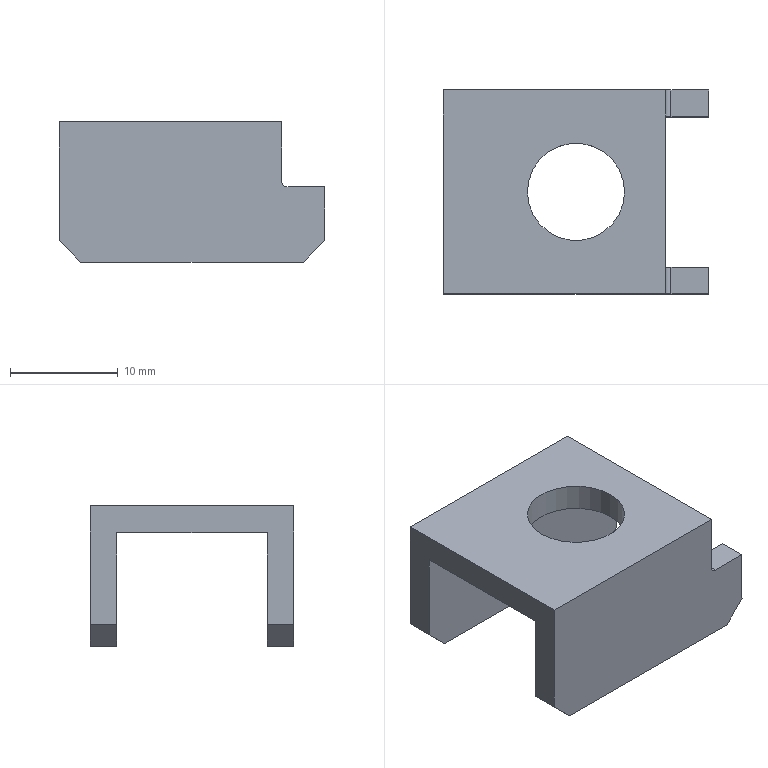Part | STEP file | gslz 2016.10.28-6_id814_x_t | 1 solid | 21 faces | box 24.6 x 18.9 x 13 mm | volume 2016 mm3 | plane 18 | cylinder 3 | commonest cylinder face diameters 1 x2 9 x1
STEP:
#1=CARTESIAN_POINT('',(165.6,245.,127.492));
#2=VERTEX_POINT('',#1);
#3=CARTESIAN_POINT('',(161.1,245.,127.492));
#4=DIRECTION('',(0.,0.,-1.));
#5=DIRECTION('',(1.,0.,0.));
#6=AXIS2_PLACEMENT_3D('',#3,#4,#5);
#7=CIRCLE('',#6,4.5);
#8=EDGE_CURVE('',#2,#2,#7,.T.);
#9=ORIENTED_EDGE('',*,*,#8,.T.);
#10=EDGE_LOOP('',(#9));
#11=FACE_BOUND('',#10,.T.);
#12=CARTESIAN_POINT('',(156.6,245.,129.992));
#13=VERTEX_POINT('',#12);
#14=CARTESIAN_POINT('',(161.1,245.,129.992));
#15=DIRECTION('',(0.,0.,-1.));
#16=DIRECTION('',(-1.,0.,0.));
#17=AXIS2_PLACEMENT_3D('',#14,#15,#16);
#18=CIRCLE('',#17,4.5);
#19=EDGE_CURVE('',#13,#13,#18,.T.);
#20=ORIENTED_EDGE('',*,*,#19,.F.);
#21=EDGE_LOOP('',(#20));
#22=FACE_BOUND('',#21,.T.);
#23=CARTESIAN_POINT('',(161.1,245.,233.066));
#24=DIRECTION('',(0.,0.,-1.));
#25=DIRECTION('',(-1.,0.,0.));
#26=AXIS2_PLACEMENT_3D('',#23,#24,#25);
#27=CYLINDRICAL_SURFACE('',#26,4.5);
#28=ADVANCED_FACE('',(#11,#22),#27,.F.);
#29=ORIENTED_EDGE('',*,*,#8,.F.);
#30=EDGE_LOOP('',(#29));
#31=FACE_BOUND('',#30,.T.);
#32=CARTESIAN_POINT('',(148.8,251.95,127.492));
#33=VERTEX_POINT('',#32);
#34=CARTESIAN_POINT('',(169.4,251.95,127.492));
#35=VERTEX_POINT('',#34);
#36=CARTESIAN_POINT('',(148.8,251.95,127.492));
#37=DIRECTION('',(1.,0.,0.));
#38=VECTOR('',#37,1.);
#39=LINE('',#36,#38);
#40=EDGE_CURVE('',#33,#35,#39,.T.);
#41=ORIENTED_EDGE('',*,*,#40,.T.);
#42=CARTESIAN_POINT('',(169.4,238.05,127.492));
#43=VERTEX_POINT('',#42);
#44=CARTESIAN_POINT('',(169.4,224.55,127.492));
#45=DIRECTION('',(0.,-1.,0.));
#46=VECTOR('',#45,1.);
#47=LINE('',#44,#46);
#48=EDGE_CURVE('',#35,#43,#47,.T.);
#49=ORIENTED_EDGE('',*,*,#48,.T.);
#50=CARTESIAN_POINT('',(148.8,238.05,127.492));
#51=VERTEX_POINT('',#50);
#52=CARTESIAN_POINT('',(173.4,238.05,127.492));
#53=DIRECTION('',(-1.,0.,0.));
#54=VECTOR('',#53,1.);
#55=LINE('',#52,#54);
#56=EDGE_CURVE('',#43,#51,#55,.T.);
#57=ORIENTED_EDGE('',*,*,#56,.T.);
#58=CARTESIAN_POINT('',(148.8,238.05,127.492));
#59=DIRECTION('',(0.,1.,0.));
#60=VECTOR('',#59,1.);
#61=LINE('',#58,#60);
#62=EDGE_CURVE('',#51,#33,#61,.T.);
#63=ORIENTED_EDGE('',*,*,#62,.T.);
#64=EDGE_LOOP('',(#41,#49,#57,#63));
#65=FACE_BOUND('',#64,.T.);
#66=CARTESIAN_POINT('',(173.4,251.95,127.492));
#67=DIRECTION('',(0.,0.,1.));
#68=DIRECTION('',(-1.,0.,0.));
#69=AXIS2_PLACEMENT_3D('',#66,#67,#68);
#70=PLANE('',#69);
#71=ADVANCED_FACE('',(#31,#65),#70,.F.);
#72=CARTESIAN_POINT('',(148.8,254.45,129.992));
#73=VERTEX_POINT('',#72);
#74=CARTESIAN_POINT('',(169.4,254.45,129.992));
#75=VERTEX_POINT('',#74);
#76=CARTESIAN_POINT('',(151.8,254.45,129.992));
#77=DIRECTION('',(1.,0.,0.));
#78=VECTOR('',#77,1.);
#79=LINE('',#76,#78);
#80=EDGE_CURVE('',#73,#75,#79,.T.);
#81=ORIENTED_EDGE('',*,*,#80,.F.);
#82=CARTESIAN_POINT('',(148.8,235.55,129.992));
#83=VERTEX_POINT('',#82);
#84=CARTESIAN_POINT('',(148.8,224.55,129.992));
#85=DIRECTION('',(0.,1.,0.));
#86=VECTOR('',#85,1.);
#87=LINE('',#84,#86);
#88=EDGE_CURVE('',#83,#73,#87,.T.);
#89=ORIENTED_EDGE('',*,*,#88,.F.);
#90=CARTESIAN_POINT('',(169.4,235.55,129.992));
#91=VERTEX_POINT('',#90);
#92=CARTESIAN_POINT('',(151.8,235.55,129.992));
#93=DIRECTION('',(-1.,0.,0.));
#94=VECTOR('',#93,1.);
#95=LINE('',#92,#94);
#96=EDGE_CURVE('',#91,#83,#95,.T.);
#97=ORIENTED_EDGE('',*,*,#96,.F.);
#98=CARTESIAN_POINT('',(169.4,224.55,129.992));
#99=DIRECTION('',(0.,1.,0.));
#100=VECTOR('',#99,1.);
#101=LINE('',#98,#100);
#102=EDGE_CURVE('',#91,#75,#101,.T.);
#103=ORIENTED_EDGE('',*,*,#102,.T.);
#104=EDGE_LOOP('',(#81,#89,#97,#103));
#105=FACE_BOUND('',#104,.T.);
#106=ORIENTED_EDGE('',*,*,#19,.T.);
#107=EDGE_LOOP('',(#106));
#108=FACE_BOUND('',#107,.T.);
#109=CARTESIAN_POINT('',(151.8,224.55,129.992));
#110=DIRECTION('',(0.,0.,-1.));
#111=DIRECTION('',(1.,0.,0.));
#112=AXIS2_PLACEMENT_3D('',#109,#110,#111);
#113=PLANE('',#112);
#114=ADVANCED_FACE('',(#105,#108),#113,.F.);
#115=CARTESIAN_POINT('',(169.4,251.95,124.492));
#116=VERTEX_POINT('',#115);
#117=CARTESIAN_POINT('',(169.4,251.95,129.992));
#118=DIRECTION('',(0.,0.,-1.));
#119=VECTOR('',#118,1.);
#120=LINE('',#117,#119);
#121=EDGE_CURVE('',#35,#116,#120,.T.);
#122=ORIENTED_EDGE('',*,*,#121,.T.);
#123=CARTESIAN_POINT('',(169.4,254.45,124.492));
#124=VERTEX_POINT('',#123);
#125=CARTESIAN_POINT('',(169.4,224.55,124.492));
#126=DIRECTION('',(0.,1.,0.));
#127=VECTOR('',#126,1.);
#128=LINE('',#125,#127);
#129=EDGE_CURVE('',#116,#124,#128,.T.);
#130=ORIENTED_EDGE('',*,*,#129,.T.);
#131=CARTESIAN_POINT('',(169.4,254.45,129.992));
#132=DIRECTION('',(0.,0.,-1.));
#133=VECTOR('',#132,1.);
#134=LINE('',#131,#133);
#135=EDGE_CURVE('',#75,#124,#134,.T.);
#136=ORIENTED_EDGE('',*,*,#135,.F.);
#137=ORIENTED_EDGE('',*,*,#102,.F.);
#138=CARTESIAN_POINT('',(169.4,235.55,124.492));
#139=VERTEX_POINT('',#138);
#140=CARTESIAN_POINT('',(169.4,235.55,129.992));
#141=DIRECTION('',(0.,0.,1.));
#142=VECTOR('',#141,1.);
#143=LINE('',#140,#142);
#144=EDGE_CURVE('',#139,#91,#143,.T.);
#145=ORIENTED_EDGE('',*,*,#144,.F.);
#146=CARTESIAN_POINT('',(169.4,238.05,124.492));
#147=VERTEX_POINT('',#146);
#148=CARTESIAN_POINT('',(169.4,224.55,124.492));
#149=DIRECTION('',(0.,1.,0.));
#150=VECTOR('',#149,1.);
#151=LINE('',#148,#150);
#152=EDGE_CURVE('',#139,#147,#151,.T.);
#153=ORIENTED_EDGE('',*,*,#152,.T.);
#154=CARTESIAN_POINT('',(169.4,238.05,129.992));
#155=DIRECTION('',(0.,0.,1.));
#156=VECTOR('',#155,1.);
#157=LINE('',#154,#156);
#158=EDGE_CURVE('',#147,#43,#157,.T.);
#159=ORIENTED_EDGE('',*,*,#158,.T.);
#160=ORIENTED_EDGE('',*,*,#48,.F.);
#161=EDGE_LOOP('',(#122,#130,#136,#137,#145,#153,#159,#160));
#162=FACE_OUTER_BOUND('',#161,.T.);
#163=CARTESIAN_POINT('',(169.4,224.55,129.992));
#164=DIRECTION('',(-1.,0.,0.));
#165=DIRECTION('',(0.,0.,-1.));
#166=AXIS2_PLACEMENT_3D('',#163,#164,#165);
#167=PLANE('',#166);
#168=ADVANCED_FACE('',(#162),#167,.F.);
#169=CARTESIAN_POINT('',(169.9,238.05,123.992));
#170=VERTEX_POINT('',#169);
#171=CARTESIAN_POINT('',(169.9,238.05,124.492));
#172=DIRECTION('',(0.,1.,0.));
#173=DIRECTION('',(1.,0.,0.));
#174=AXIS2_PLACEMENT_3D('',#171,#172,#173);
#175=CIRCLE('',#174,0.5);
#176=EDGE_CURVE('',#170,#147,#175,.T.);
#177=ORIENTED_EDGE('',*,*,#176,.T.);
#178=ORIENTED_EDGE('',*,*,#152,.F.);
#179=CARTESIAN_POINT('',(169.9,235.55,123.992));
#180=VERTEX_POINT('',#179);
#181=CARTESIAN_POINT('',(169.9,235.55,124.492));
#182=DIRECTION('',(0.,1.,0.));
#183=DIRECTION('',(1.,0.,0.));
#184=AXIS2_PLACEMENT_3D('',#181,#182,#183);
#185=CIRCLE('',#184,0.5);
#186=EDGE_CURVE('',#180,#139,#185,.T.);
#187=ORIENTED_EDGE('',*,*,#186,.F.);
#188=CARTESIAN_POINT('',(169.9,224.55,123.992));
#189=DIRECTION('',(0.,1.,0.));
#190=VECTOR('',#189,1.);
#191=LINE('',#188,#190);
#192=EDGE_CURVE('',#180,#170,#191,.T.);
#193=ORIENTED_EDGE('',*,*,#192,.T.);
#194=EDGE_LOOP('',(#177,#178,#187,#193));
#195=FACE_OUTER_BOUND('',#194,.T.);
#196=CARTESIAN_POINT('',(169.9,224.55,124.492));
#197=DIRECTION('',(0.,-1.,0.));
#198=DIRECTION('',(1.,0.,0.));
#199=AXIS2_PLACEMENT_3D('',#196,#197,#198);
#200=CYLINDRICAL_SURFACE('',#199,0.5);
#201=ADVANCED_FACE('',(#195),#200,.F.);
#202=CARTESIAN_POINT('',(169.9,251.95,123.992));
#203=VERTEX_POINT('',#202);
#204=CARTESIAN_POINT('',(169.9,251.95,124.492));
#205=DIRECTION('',(0.,-1.,0.));
#206=DIRECTION('',(-1.,0.,0.));
#207=AXIS2_PLACEMENT_3D('',#204,#205,#206);
#208=CIRCLE('',#207,0.5);
#209=EDGE_CURVE('',#116,#203,#208,.T.);
#210=ORIENTED_EDGE('',*,*,#209,.T.);
#211=CARTESIAN_POINT('',(169.9,254.45,123.992));
#212=VERTEX_POINT('',#211);
#213=CARTESIAN_POINT('',(169.9,224.55,123.992));
#214=DIRECTION('',(0.,-1.,0.));
#215=VECTOR('',#214,1.);
#216=LINE('',#213,#215);
#217=EDGE_CURVE('',#212,#203,#216,.T.);
#218=ORIENTED_EDGE('',*,*,#217,.F.);
#219=CARTESIAN_POINT('',(169.9,254.45,124.492));
#220=DIRECTION('',(0.,-1.,0.));
#221=DIRECTION('',(-1.,0.,0.));
#222=AXIS2_PLACEMENT_3D('',#219,#220,#221);
#223=CIRCLE('',#222,0.5);
#224=EDGE_CURVE('',#124,#212,#223,.T.);
#225=ORIENTED_EDGE('',*,*,#224,.F.);
#226=ORIENTED_EDGE('',*,*,#129,.F.);
#227=EDGE_LOOP('',(#210,#218,#225,#226));
#228=FACE_OUTER_BOUND('',#227,.T.);
#229=CARTESIAN_POINT('',(169.9,224.55,124.492));
#230=DIRECTION('',(0.,1.,0.));
#231=DIRECTION('',(-1.,0.,0.));
#232=AXIS2_PLACEMENT_3D('',#229,#230,#231);
#233=CYLINDRICAL_SURFACE('',#232,0.5);
#234=ADVANCED_FACE('',(#228),#233,.F.);
#235=CARTESIAN_POINT('',(148.8,254.45,118.992));
#236=VERTEX_POINT('',#235);
#237=CARTESIAN_POINT('',(148.8,254.45,49.155));
#238=DIRECTION('',(0.,0.,1.));
#239=VECTOR('',#238,1.);
#240=LINE('',#237,#239);
#241=EDGE_CURVE('',#236,#73,#240,.T.);
#242=ORIENTED_EDGE('',*,*,#241,.T.);
#243=ORIENTED_EDGE('',*,*,#80,.T.);
#244=ORIENTED_EDGE('',*,*,#135,.T.);
#245=ORIENTED_EDGE('',*,*,#224,.T.);
#246=CARTESIAN_POINT('',(173.4,254.45,123.992));
#247=VERTEX_POINT('',#246);
#248=CARTESIAN_POINT('',(173.4,254.45,123.992));
#249=DIRECTION('',(1.,0.,0.));
#250=VECTOR('',#249,1.);
#251=LINE('',#248,#250);
#252=EDGE_CURVE('',#212,#247,#251,.T.);
#253=ORIENTED_EDGE('',*,*,#252,.T.);
#254=CARTESIAN_POINT('',(173.4,254.45,118.992));
#255=VERTEX_POINT('',#254);
#256=CARTESIAN_POINT('',(173.4,254.45,49.155));
#257=DIRECTION('',(0.,0.,1.));
#258=VECTOR('',#257,1.);
#259=LINE('',#256,#258);
#260=EDGE_CURVE('',#255,#247,#259,.T.);
#261=ORIENTED_EDGE('',*,*,#260,.F.);
#262=CARTESIAN_POINT('',(171.4,254.45,116.992));
#263=VERTEX_POINT('',#262);
#264=CARTESIAN_POINT('',(173.4,254.45,118.992));
#265=DIRECTION('',(-0.7071,0.,-0.7071));
#266=VECTOR('',#265,1.);
#267=LINE('',#264,#266);
#268=EDGE_CURVE('',#255,#263,#267,.T.);
#269=ORIENTED_EDGE('',*,*,#268,.T.);
#270=CARTESIAN_POINT('',(150.8,254.45,116.992));
#271=VERTEX_POINT('',#270);
#272=CARTESIAN_POINT('',(171.4,254.45,116.992));
#273=DIRECTION('',(-1.,0.,0.));
#274=VECTOR('',#273,1.);
#275=LINE('',#272,#274);
#276=EDGE_CURVE('',#263,#271,#275,.T.);
#277=ORIENTED_EDGE('',*,*,#276,.T.);
#278=CARTESIAN_POINT('',(150.8,254.45,116.992));
#279=DIRECTION('',(-0.7071,0.,0.7071));
#280=VECTOR('',#279,1.);
#281=LINE('',#278,#280);
#282=EDGE_CURVE('',#271,#236,#281,.T.);
#283=ORIENTED_EDGE('',*,*,#282,.T.);
#284=EDGE_LOOP('',(#242,#243,#244,#245,#253,#261,#269,#277,#283));
#285=FACE_OUTER_BOUND('',#284,.T.);
#286=CARTESIAN_POINT('',(173.4,254.45,49.155));
#287=DIRECTION('',(0.,-1.,0.));
#288=DIRECTION('',(0.,0.,1.));
#289=AXIS2_PLACEMENT_3D('',#286,#287,#288);
#290=PLANE('',#289);
#291=ADVANCED_FACE('',(#285),#290,.F.);
#292=CARTESIAN_POINT('',(148.8,251.95,118.992));
#293=VERTEX_POINT('',#292);
#294=CARTESIAN_POINT('',(148.8,251.95,127.492));
#295=DIRECTION('',(0.,0.,-1.));
#296=VECTOR('',#295,1.);
#297=LINE('',#294,#296);
#298=EDGE_CURVE('',#33,#293,#297,.T.);
#299=ORIENTED_EDGE('',*,*,#298,.F.);
#300=ORIENTED_EDGE('',*,*,#62,.F.);
#301=CARTESIAN_POINT('',(148.8,238.05,118.992));
#302=VERTEX_POINT('',#301);
#303=CARTESIAN_POINT('',(148.8,238.05,127.492));
#304=DIRECTION('',(0.,0.,-1.));
#305=VECTOR('',#304,1.);
#306=LINE('',#303,#305);
#307=EDGE_CURVE('',#51,#302,#306,.T.);
#308=ORIENTED_EDGE('',*,*,#307,.T.);
#309=CARTESIAN_POINT('',(148.8,235.55,118.992));
#310=VERTEX_POINT('',#309);
#311=CARTESIAN_POINT('',(148.8,224.55,118.992));
#312=DIRECTION('',(0.,1.,0.));
#313=VECTOR('',#312,1.);
#314=LINE('',#311,#313);
#315=EDGE_CURVE('',#310,#302,#314,.T.);
#316=ORIENTED_EDGE('',*,*,#315,.F.);
#317=CARTESIAN_POINT('',(148.8,235.55,49.155));
#318=DIRECTION('',(0.,0.,1.));
#319=VECTOR('',#318,1.);
#320=LINE('',#317,#319);
#321=EDGE_CURVE('',#310,#83,#320,.T.);
#322=ORIENTED_EDGE('',*,*,#321,.T.);
#323=ORIENTED_EDGE('',*,*,#88,.T.);
#324=ORIENTED_EDGE('',*,*,#241,.F.);
#325=CARTESIAN_POINT('',(148.8,224.55,118.992));
#326=DIRECTION('',(0.,1.,0.));
#327=VECTOR('',#326,1.);
#328=LINE('',#325,#327);
#329=EDGE_CURVE('',#293,#236,#328,.T.);
#330=ORIENTED_EDGE('',*,*,#329,.F.);
#331=EDGE_LOOP('',(#299,#300,#308,#316,#322,#323,#324,#330));
#332=FACE_OUTER_BOUND('',#331,.T.);
#333=CARTESIAN_POINT('',(148.8,224.55,119.992));
#334=DIRECTION('',(1.,0.,0.));
#335=DIRECTION('',(0.,0.,1.));
#336=AXIS2_PLACEMENT_3D('',#333,#334,#335);
#337=PLANE('',#336);
#338=ADVANCED_FACE('',(#332),#337,.F.);
#339=ORIENTED_EDGE('',*,*,#307,.F.);
#340=ORIENTED_EDGE('',*,*,#56,.F.);
#341=ORIENTED_EDGE('',*,*,#158,.F.);
#342=ORIENTED_EDGE('',*,*,#176,.F.);
#343=CARTESIAN_POINT('',(173.4,238.05,123.992));
#344=VERTEX_POINT('',#343);
#345=CARTESIAN_POINT('',(169.9,238.05,123.992));
#346=DIRECTION('',(-1.,0.,0.));
#347=VECTOR('',#346,1.);
#348=LINE('',#345,#347);
#349=EDGE_CURVE('',#344,#170,#348,.T.);
#350=ORIENTED_EDGE('',*,*,#349,.F.);
#351=CARTESIAN_POINT('',(173.4,238.05,118.992));
#352=VERTEX_POINT('',#351);
#353=CARTESIAN_POINT('',(173.4,238.05,127.492));
#354=DIRECTION('',(0.,0.,-1.));
#355=VECTOR('',#354,1.);
#356=LINE('',#353,#355);
#357=EDGE_CURVE('',#344,#352,#356,.T.);
#358=ORIENTED_EDGE('',*,*,#357,.T.);
#359=CARTESIAN_POINT('',(171.4,238.05,116.992));
#360=VERTEX_POINT('',#359);
#361=CARTESIAN_POINT('',(173.4,238.05,118.992));
#362=DIRECTION('',(0.7071,0.,0.7071));
#363=VECTOR('',#362,1.);
#364=LINE('',#361,#363);
#365=EDGE_CURVE('',#360,#352,#364,.T.);
#366=ORIENTED_EDGE('',*,*,#365,.F.);
#367=CARTESIAN_POINT('',(150.8,238.05,116.992));
#368=VERTEX_POINT('',#367);
#369=CARTESIAN_POINT('',(171.4,238.05,116.992));
#370=DIRECTION('',(1.,0.,0.));
#371=VECTOR('',#370,1.);
#372=LINE('',#369,#371);
#373=EDGE_CURVE('',#368,#360,#372,.T.);
#374=ORIENTED_EDGE('',*,*,#373,.F.);
#375=CARTESIAN_POINT('',(150.8,238.05,116.992));
#376=DIRECTION('',(0.7071,0.,-0.7071));
#377=VECTOR('',#376,1.);
#378=LINE('',#375,#377);
#379=EDGE_CURVE('',#302,#368,#378,.T.);
#380=ORIENTED_EDGE('',*,*,#379,.F.);
#381=EDGE_LOOP('',(#339,#340,#341,#342,#350,#358,#366,#374,#380));
#382=FACE_OUTER_BOUND('',#381,.T.);
#383=CARTESIAN_POINT('',(173.4,238.05,127.492));
#384=DIRECTION('',(0.,1.,0.));
#385=DIRECTION('',(0.,0.,-1.));
#386=AXIS2_PLACEMENT_3D('',#383,#384,#385);
#387=PLANE('',#386);
#388=ADVANCED_FACE('',(#382),#387,.T.);
#389=ORIENTED_EDGE('',*,*,#186,.T.);
#390=ORIENTED_EDGE('',*,*,#144,.T.);
#391=ORIENTED_EDGE('',*,*,#96,.T.);
#392=ORIENTED_EDGE('',*,*,#321,.F.);
#393=CARTESIAN_POINT('',(150.8,235.55,116.992));
#394=VERTEX_POINT('',#393);
#395=CARTESIAN_POINT('',(150.8,235.55,116.992));
#396=DIRECTION('',(0.7071,0.,-0.7071));
#397=VECTOR('',#396,1.);
#398=LINE('',#395,#397);
#399=EDGE_CURVE('',#310,#394,#398,.T.);
#400=ORIENTED_EDGE('',*,*,#399,.T.);
#401=CARTESIAN_POINT('',(171.4,235.55,116.992));
#402=VERTEX_POINT('',#401);
#403=CARTESIAN_POINT('',(171.4,235.55,116.992));
#404=DIRECTION('',(1.,0.,0.));
#405=VECTOR('',#404,1.);
#406=LINE('',#403,#405);
#407=EDGE_CURVE('',#394,#402,#406,.T.);
#408=ORIENTED_EDGE('',*,*,#407,.T.);
#409=CARTESIAN_POINT('',(173.4,235.55,118.992));
#410=VERTEX_POINT('',#409);
#411=CARTESIAN_POINT('',(173.4,235.55,118.992));
#412=DIRECTION('',(0.7071,0.,0.7071));
#413=VECTOR('',#412,1.);
#414=LINE('',#411,#413);
#415=EDGE_CURVE('',#402,#410,#414,.T.);
#416=ORIENTED_EDGE('',*,*,#415,.T.);
#417=CARTESIAN_POINT('',(173.4,235.55,123.992));
#418=VERTEX_POINT('',#417);
#419=CARTESIAN_POINT('',(173.4,235.55,49.155));
#420=DIRECTION('',(0.,0.,1.));
#421=VECTOR('',#420,1.);
#422=LINE('',#419,#421);
#423=EDGE_CURVE('',#410,#418,#422,.T.);
#424=ORIENTED_EDGE('',*,*,#423,.T.);
#425=CARTESIAN_POINT('',(169.9,235.55,123.992));
#426=DIRECTION('',(-1.,0.,0.));
#427=VECTOR('',#426,1.);
#428=LINE('',#425,#427);
#429=EDGE_CURVE('',#418,#180,#428,.T.);
#430=ORIENTED_EDGE('',*,*,#429,.T.);
#431=EDGE_LOOP('',(#389,#390,#391,#392,#400,#408,#416,#424,#430));
#432=FACE_OUTER_BOUND('',#431,.T.);
#433=CARTESIAN_POINT('',(148.8,235.55,49.155));
#434=DIRECTION('',(0.,1.,0.));
#435=DIRECTION('',(0.,0.,-1.));
#436=AXIS2_PLACEMENT_3D('',#433,#434,#435);
#437=PLANE('',#436);
#438=ADVANCED_FACE('',(#432),#437,.F.);
#439=ORIENTED_EDGE('',*,*,#209,.F.);
#440=ORIENTED_EDGE('',*,*,#121,.F.);
#441=ORIENTED_EDGE('',*,*,#40,.F.);
#442=ORIENTED_EDGE('',*,*,#298,.T.);
#443=CARTESIAN_POINT('',(150.8,251.95,116.992));
#444=VERTEX_POINT('',#443);
#445=CARTESIAN_POINT('',(150.8,251.95,116.992));
#446=DIRECTION('',(-0.7071,0.,0.7071));
#447=VECTOR('',#446,1.);
#448=LINE('',#445,#447);
#449=EDGE_CURVE('',#444,#293,#448,.T.);
#450=ORIENTED_EDGE('',*,*,#449,.F.);
#451=CARTESIAN_POINT('',(171.4,251.95,116.992));
#452=VERTEX_POINT('',#451);
#453=CARTESIAN_POINT('',(171.4,251.95,116.992));
#454=DIRECTION('',(-1.,0.,0.));
#455=VECTOR('',#454,1.);
#456=LINE('',#453,#455);
#457=EDGE_CURVE('',#452,#444,#456,.T.);
#458=ORIENTED_EDGE('',*,*,#457,.F.);
#459=CARTESIAN_POINT('',(173.4,251.95,118.992));
#460=VERTEX_POINT('',#459);
#461=CARTESIAN_POINT('',(173.4,251.95,118.992));
#462=DIRECTION('',(-0.7071,0.,-0.7071));
#463=VECTOR('',#462,1.);
#464=LINE('',#461,#463);
#465=EDGE_CURVE('',#460,#452,#464,.T.);
#466=ORIENTED_EDGE('',*,*,#465,.F.);
#467=CARTESIAN_POINT('',(173.4,251.95,123.992));
#468=VERTEX_POINT('',#467);
#469=CARTESIAN_POINT('',(173.4,251.95,127.492));
#470=DIRECTION('',(0.,0.,-1.));
#471=VECTOR('',#470,1.);
#472=LINE('',#469,#471);
#473=EDGE_CURVE('',#468,#460,#472,.T.);
#474=ORIENTED_EDGE('',*,*,#473,.F.);
#475=CARTESIAN_POINT('',(169.9,251.95,123.992));
#476=DIRECTION('',(1.,0.,0.));
#477=VECTOR('',#476,1.);
#478=LINE('',#475,#477);
#479=EDGE_CURVE('',#203,#468,#478,.T.);
#480=ORIENTED_EDGE('',*,*,#479,.F.);
#481=EDGE_LOOP('',(#439,#440,#441,#442,#450,#458,#466,#474,#480));
#482=FACE_OUTER_BOUND('',#481,.T.);
#483=CARTESIAN_POINT('',(148.8,251.95,127.492));
#484=DIRECTION('',(0.,-1.,0.));
#485=DIRECTION('',(0.,0.,1.));
#486=AXIS2_PLACEMENT_3D('',#483,#484,#485);
#487=PLANE('',#486);
#488=ADVANCED_FACE('',(#482),#487,.T.);
#489=ORIENTED_EDGE('',*,*,#457,.T.);
#490=CARTESIAN_POINT('',(150.8,224.55,116.992));
#491=DIRECTION('',(0.,1.,0.));
#492=VECTOR('',#491,1.);
#493=LINE('',#490,#492);
#494=EDGE_CURVE('',#444,#271,#493,.T.);
#495=ORIENTED_EDGE('',*,*,#494,.T.);
#496=ORIENTED_EDGE('',*,*,#276,.F.);
#497=CARTESIAN_POINT('',(171.4,224.55,116.992));
#498=DIRECTION('',(0.,1.,0.));
#499=VECTOR('',#498,1.);
#500=LINE('',#497,#499);
#501=EDGE_CURVE('',#452,#263,#500,.T.);
#502=ORIENTED_EDGE('',*,*,#501,.F.);
#503=EDGE_LOOP('',(#489,#495,#496,#502));
#504=FACE_OUTER_BOUND('',#503,.T.);
#505=CARTESIAN_POINT('',(171.4,224.55,116.992));
#506=DIRECTION('',(0.,0.,1.));
#507=DIRECTION('',(-1.,0.,0.));
#508=AXIS2_PLACEMENT_3D('',#505,#506,#507);
#509=PLANE('',#508);
#510=ADVANCED_FACE('',(#504),#509,.F.);
#511=ORIENTED_EDGE('',*,*,#449,.T.);
#512=ORIENTED_EDGE('',*,*,#329,.T.);
#513=ORIENTED_EDGE('',*,*,#282,.F.);
#514=ORIENTED_EDGE('',*,*,#494,.F.);
#515=EDGE_LOOP('',(#511,#512,#513,#514));
#516=FACE_OUTER_BOUND('',#515,.T.);
#517=CARTESIAN_POINT('',(150.8,224.55,116.992));
#518=DIRECTION('',(0.7071,0.,0.7071));
#519=DIRECTION('',(-0.7071,0.,0.7071));
#520=AXIS2_PLACEMENT_3D('',#517,#518,#519);
#521=PLANE('',#520);
#522=ADVANCED_FACE('',(#516),#521,.F.);
#523=ORIENTED_EDGE('',*,*,#465,.T.);
#524=ORIENTED_EDGE('',*,*,#501,.T.);
#525=ORIENTED_EDGE('',*,*,#268,.F.);
#526=CARTESIAN_POINT('',(173.4,224.55,118.992));
#527=DIRECTION('',(0.,1.,0.));
#528=VECTOR('',#527,1.);
#529=LINE('',#526,#528);
#530=EDGE_CURVE('',#460,#255,#529,.T.);
#531=ORIENTED_EDGE('',*,*,#530,.F.);
#532=EDGE_LOOP('',(#523,#524,#525,#531));
#533=FACE_OUTER_BOUND('',#532,.T.);
#534=CARTESIAN_POINT('',(173.4,224.55,118.992));
#535=DIRECTION('',(-0.7071,0.,0.7071));
#536=DIRECTION('',(0.7071,0.,0.7071));
#537=AXIS2_PLACEMENT_3D('',#534,#535,#536);
#538=PLANE('',#537);
#539=ADVANCED_FACE('',(#533),#538,.F.);
#540=ORIENTED_EDGE('',*,*,#473,.T.);
#541=ORIENTED_EDGE('',*,*,#530,.T.);
#542=ORIENTED_EDGE('',*,*,#260,.T.);
#543=CARTESIAN_POINT('',(173.4,224.55,123.992));
#544=DIRECTION('',(0.,1.,0.));
#545=VECTOR('',#544,1.);
#546=LINE('',#543,#545);
#547=EDGE_CURVE('',#468,#247,#546,.T.);
#548=ORIENTED_EDGE('',*,*,#547,.F.);
#549=EDGE_LOOP('',(#540,#541,#542,#548));
#550=FACE_OUTER_BOUND('',#549,.T.);
#551=CARTESIAN_POINT('',(173.4,224.55,123.992));
#552=DIRECTION('',(-1.,0.,0.));
#553=DIRECTION('',(0.,0.,-1.));
#554=AXIS2_PLACEMENT_3D('',#551,#552,#553);
#555=PLANE('',#554);
#556=ADVANCED_FACE('',(#550),#555,.F.);
#557=ORIENTED_EDGE('',*,*,#217,.T.);
#558=ORIENTED_EDGE('',*,*,#479,.T.);
#559=ORIENTED_EDGE('',*,*,#547,.T.);
#560=ORIENTED_EDGE('',*,*,#252,.F.);
#561=EDGE_LOOP('',(#557,#558,#559,#560));
#562=FACE_OUTER_BOUND('',#561,.T.);
#563=CARTESIAN_POINT('',(169.9,224.55,123.992));
#564=DIRECTION('',(0.,0.,-1.));
#565=DIRECTION('',(1.,0.,0.));
#566=AXIS2_PLACEMENT_3D('',#563,#564,#565);
#567=PLANE('',#566);
#568=ADVANCED_FACE('',(#562),#567,.F.);
#569=ORIENTED_EDGE('',*,*,#429,.F.);
#570=CARTESIAN_POINT('',(173.4,224.55,123.992));
#571=DIRECTION('',(0.,1.,0.));
#572=VECTOR('',#571,1.);
#573=LINE('',#570,#572);
#574=EDGE_CURVE('',#418,#344,#573,.T.);
#575=ORIENTED_EDGE('',*,*,#574,.T.);
#576=ORIENTED_EDGE('',*,*,#349,.T.);
#577=ORIENTED_EDGE('',*,*,#192,.F.);
#578=EDGE_LOOP('',(#569,#575,#576,#577));
#579=FACE_OUTER_BOUND('',#578,.T.);
#580=CARTESIAN_POINT('',(169.9,224.55,123.992));
#581=DIRECTION('',(0.,0.,-1.));
#582=DIRECTION('',(-1.,0.,0.));
#583=AXIS2_PLACEMENT_3D('',#580,#581,#582);
#584=PLANE('',#583);
#585=ADVANCED_FACE('',(#579),#584,.F.);
#586=ORIENTED_EDGE('',*,*,#373,.T.);
#587=CARTESIAN_POINT('',(171.4,224.55,116.992));
#588=DIRECTION('',(0.,1.,0.));
#589=VECTOR('',#588,1.);
#590=LINE('',#587,#589);
#591=EDGE_CURVE('',#402,#360,#590,.T.);
#592=ORIENTED_EDGE('',*,*,#591,.F.);
#593=ORIENTED_EDGE('',*,*,#407,.F.);
#594=CARTESIAN_POINT('',(150.8,224.55,116.992));
#595=DIRECTION('',(0.,1.,0.));
#596=VECTOR('',#595,1.);
#597=LINE('',#594,#596);
#598=EDGE_CURVE('',#394,#368,#597,.T.);
#599=ORIENTED_EDGE('',*,*,#598,.T.);
#600=EDGE_LOOP('',(#586,#592,#593,#599));
#601=FACE_OUTER_BOUND('',#600,.T.);
#602=CARTESIAN_POINT('',(171.4,224.55,116.992));
#603=DIRECTION('',(0.,0.,1.));
#604=DIRECTION('',(-1.,0.,0.));
#605=AXIS2_PLACEMENT_3D('',#602,#603,#604);
#606=PLANE('',#605);
#607=ADVANCED_FACE('',(#601),#606,.F.);
#608=ORIENTED_EDGE('',*,*,#379,.T.);
#609=ORIENTED_EDGE('',*,*,#598,.F.);
#610=ORIENTED_EDGE('',*,*,#399,.F.);
#611=ORIENTED_EDGE('',*,*,#315,.T.);
#612=EDGE_LOOP('',(#608,#609,#610,#611));
#613=FACE_OUTER_BOUND('',#612,.T.);
#614=CARTESIAN_POINT('',(150.8,224.55,116.992));
#615=DIRECTION('',(0.7071,0.,0.7071));
#616=DIRECTION('',(-0.7071,0.,0.7071));
#617=AXIS2_PLACEMENT_3D('',#614,#615,#616);
#618=PLANE('',#617);
#619=ADVANCED_FACE('',(#613),#618,.F.);
#620=ORIENTED_EDGE('',*,*,#365,.T.);
#621=CARTESIAN_POINT('',(173.4,224.55,118.992));
#622=DIRECTION('',(0.,1.,0.));
#623=VECTOR('',#622,1.);
#624=LINE('',#621,#623);
#625=EDGE_CURVE('',#410,#352,#624,.T.);
#626=ORIENTED_EDGE('',*,*,#625,.F.);
#627=ORIENTED_EDGE('',*,*,#415,.F.);
#628=ORIENTED_EDGE('',*,*,#591,.T.);
#629=EDGE_LOOP('',(#620,#626,#627,#628));
#630=FACE_OUTER_BOUND('',#629,.T.);
#631=CARTESIAN_POINT('',(173.4,224.55,118.992));
#632=DIRECTION('',(-0.7071,0.,0.7071));
#633=DIRECTION('',(0.7071,0.,0.7071));
#634=AXIS2_PLACEMENT_3D('',#631,#632,#633);
#635=PLANE('',#634);
#636=ADVANCED_FACE('',(#630),#635,.F.);
#637=ORIENTED_EDGE('',*,*,#357,.F.);
#638=ORIENTED_EDGE('',*,*,#574,.F.);
#639=ORIENTED_EDGE('',*,*,#423,.F.);
#640=ORIENTED_EDGE('',*,*,#625,.T.);
#641=EDGE_LOOP('',(#637,#638,#639,#640));
#642=FACE_OUTER_BOUND('',#641,.T.);
#643=CARTESIAN_POINT('',(173.4,224.55,123.992));
#644=DIRECTION('',(-1.,0.,0.));
#645=DIRECTION('',(0.,0.,-1.));
#646=AXIS2_PLACEMENT_3D('',#643,#644,#645);
#647=PLANE('',#646);
#648=ADVANCED_FACE('',(#642),#647,.F.);
#649=CLOSED_SHELL('',(#28,#71,#114,#168,#201,#234,#291,#338,#388,#438,#488,#510,#522,#539,#556,#568,#585,#607,#619,#636,#648));
#650=MANIFOLD_SOLID_BREP('',#649);
#651=(LENGTH_UNIT()NAMED_UNIT(*)SI_UNIT(.MILLI.,.METRE.));
#652=UNCERTAINTY_MEASURE_WITH_UNIT(LENGTH_MEASURE(0.00002),#651,'','');
#653=(NAMED_UNIT(*)PLANE_ANGLE_UNIT()SI_UNIT($,.RADIAN.));
#654=PLANE_ANGLE_MEASURE_WITH_UNIT(PLANE_ANGLE_MEASURE(0.01745),#653);
#655=DIMENSIONAL_EXPONENTS(0.,0.,0.,0.,0.,0.,0.);
#656=(CONVERSION_BASED_UNIT('DEGREE',#654)NAMED_UNIT(#655)PLANE_ANGLE_UNIT());
#657=(NAMED_UNIT(*)SI_UNIT($,.STERADIAN.)SOLID_ANGLE_UNIT());
#658=(GEOMETRIC_REPRESENTATION_CONTEXT(3)GLOBAL_UNCERTAINTY_ASSIGNED_CONTEXT((#652))GLOBAL_UNIT_ASSIGNED_CONTEXT((#651,#656,#657))REPRESENTATION_CONTEXT('',''));
#659=ADVANCED_BREP_SHAPE_REPRESENTATION('',(#650),#658);